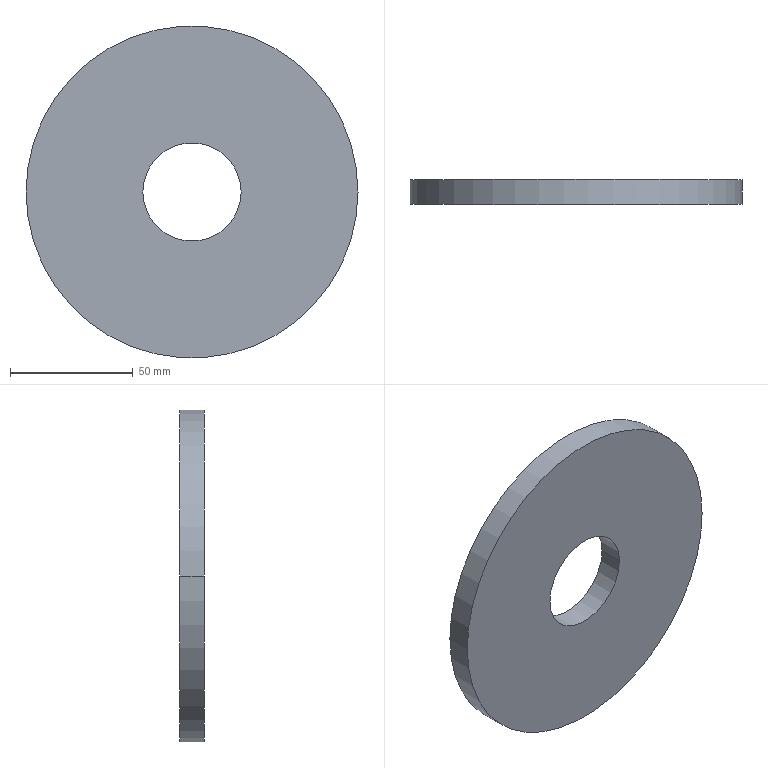Part | SolidWorks | features BaseBody 1 | 1 solid | 6 faces | box 135 x 10 x 135 mm | volume 130572 mm3 | cylinder 4 | plane 2 | commonest cylinder face diameters 40 x2 135 x2
STEP:
#1=CARTESIAN_POINT('',(-2112.95,1114.894,-1577.624));
#2=VERTEX_POINT('',#1);
#3=CARTESIAN_POINT('',(-2112.95,1104.894,-1577.624));
#4=VERTEX_POINT('',#3);
#5=CARTESIAN_POINT('',(-2112.95,1114.894,-1577.624));
#6=DIRECTION('',(0.,-1.,0.));
#7=VECTOR('',#6,1000.);
#8=LINE('',#5,#7);
#9=EDGE_CURVE('',#2,#4,#8,.T.);
#10=ORIENTED_EDGE('',*,*,#9,.F.);
#11=CARTESIAN_POINT('',(-2152.95,1114.894,-1577.624));
#12=VERTEX_POINT('',#11);
#13=CARTESIAN_POINT('',(-2132.95,1114.894,-1577.624));
#14=DIRECTION('',(0.,1.,0.));
#15=DIRECTION('',(1.,0.,0.));
#16=AXIS2_PLACEMENT_3D('',#13,#14,#15);
#17=CIRCLE('',#16,20.);
#18=EDGE_CURVE('',#2,#12,#17,.T.);
#19=ORIENTED_EDGE('',*,*,#18,.T.);
#20=CARTESIAN_POINT('',(-2152.95,1104.894,-1577.624));
#21=VERTEX_POINT('',#20);
#22=CARTESIAN_POINT('',(-2152.95,1114.894,-1577.624));
#23=DIRECTION('',(0.,-1.,0.));
#24=VECTOR('',#23,1000.);
#25=LINE('',#22,#24);
#26=EDGE_CURVE('',#12,#21,#25,.T.);
#27=ORIENTED_EDGE('',*,*,#26,.T.);
#28=CARTESIAN_POINT('',(-2132.95,1104.894,-1577.624));
#29=DIRECTION('',(0.,-1.,0.));
#30=DIRECTION('',(-1.,0.,0.));
#31=AXIS2_PLACEMENT_3D('',#28,#29,#30);
#32=CIRCLE('',#31,20.);
#33=EDGE_CURVE('',#21,#4,#32,.T.);
#34=ORIENTED_EDGE('',*,*,#33,.T.);
#35=EDGE_LOOP('',(#10,#19,#27,#34));
#36=FACE_OUTER_BOUND('',#35,.T.);
#37=CARTESIAN_POINT('',(-2132.95,1114.894,-1577.624));
#38=DIRECTION('',(0.,1.,0.));
#39=DIRECTION('',(1.,0.,0.));
#40=AXIS2_PLACEMENT_3D('',#37,#38,#39);
#41=CYLINDRICAL_SURFACE('',#40,20.);
#42=ADVANCED_FACE('',(#36),#41,.F.);
#43=CARTESIAN_POINT('',(-2065.45,1104.894,-1577.624));
#44=VERTEX_POINT('',#43);
#45=CARTESIAN_POINT('',(-2065.45,1114.894,-1577.624));
#46=VERTEX_POINT('',#45);
#47=CARTESIAN_POINT('',(-2065.45,1104.894,-1577.624));
#48=DIRECTION('',(0.,1.,0.));
#49=VECTOR('',#48,1000.);
#50=LINE('',#47,#49);
#51=EDGE_CURVE('',#44,#46,#50,.T.);
#52=ORIENTED_EDGE('',*,*,#51,.F.);
#53=CARTESIAN_POINT('',(-2200.45,1104.894,-1577.624));
#54=VERTEX_POINT('',#53);
#55=CARTESIAN_POINT('',(-2132.95,1104.894,-1577.624));
#56=DIRECTION('',(0.,-1.,0.));
#57=DIRECTION('',(-1.,0.,0.));
#58=AXIS2_PLACEMENT_3D('',#55,#56,#57);
#59=CIRCLE('',#58,67.5);
#60=EDGE_CURVE('',#54,#44,#59,.T.);
#61=ORIENTED_EDGE('',*,*,#60,.F.);
#62=CARTESIAN_POINT('',(-2200.45,1114.894,-1577.624));
#63=VERTEX_POINT('',#62);
#64=CARTESIAN_POINT('',(-2200.45,1104.894,-1577.624));
#65=DIRECTION('',(0.,1.,0.));
#66=VECTOR('',#65,1000.);
#67=LINE('',#64,#66);
#68=EDGE_CURVE('',#54,#63,#67,.T.);
#69=ORIENTED_EDGE('',*,*,#68,.T.);
#70=CARTESIAN_POINT('',(-2132.95,1114.894,-1577.624));
#71=DIRECTION('',(0.,1.,0.));
#72=DIRECTION('',(1.,0.,0.));
#73=AXIS2_PLACEMENT_3D('',#70,#71,#72);
#74=CIRCLE('',#73,67.5);
#75=EDGE_CURVE('',#46,#63,#74,.T.);
#76=ORIENTED_EDGE('',*,*,#75,.F.);
#77=EDGE_LOOP('',(#52,#61,#69,#76));
#78=FACE_OUTER_BOUND('',#77,.T.);
#79=CARTESIAN_POINT('',(-2132.95,1104.894,-1577.624));
#80=DIRECTION('',(0.,1.,0.));
#81=DIRECTION('',(1.,0.,0.));
#82=AXIS2_PLACEMENT_3D('',#79,#80,#81);
#83=CYLINDRICAL_SURFACE('',#82,67.5);
#84=ADVANCED_FACE('',(#78),#83,.T.);
#85=ORIENTED_EDGE('',*,*,#33,.F.);
#86=CARTESIAN_POINT('',(-2132.95,1104.894,-1577.624));
#87=DIRECTION('',(0.,-1.,0.));
#88=DIRECTION('',(1.,0.,0.));
#89=AXIS2_PLACEMENT_3D('',#86,#87,#88);
#90=CIRCLE('',#89,20.);
#91=EDGE_CURVE('',#4,#21,#90,.T.);
#92=ORIENTED_EDGE('',*,*,#91,.F.);
#93=EDGE_LOOP('',(#85,#92));
#94=FACE_BOUND('',#93,.T.);
#95=ORIENTED_EDGE('',*,*,#60,.T.);
#96=CARTESIAN_POINT('',(-2132.95,1104.894,-1577.624));
#97=DIRECTION('',(0.,-1.,0.));
#98=DIRECTION('',(1.,0.,0.));
#99=AXIS2_PLACEMENT_3D('',#96,#97,#98);
#100=CIRCLE('',#99,67.5);
#101=EDGE_CURVE('',#44,#54,#100,.T.);
#102=ORIENTED_EDGE('',*,*,#101,.T.);
#103=EDGE_LOOP('',(#95,#102));
#104=FACE_OUTER_BOUND('',#103,.T.);
#105=CARTESIAN_POINT('',(-2064.1,1104.894,-1646.474));
#106=DIRECTION('',(0.,-1.,0.));
#107=DIRECTION('',(0.,0.,-1.));
#108=AXIS2_PLACEMENT_3D('',#105,#106,#107);
#109=PLANE('',#108);
#110=ADVANCED_FACE('',(#94,#104),#109,.T.);
#111=ORIENTED_EDGE('',*,*,#91,.T.);
#112=ORIENTED_EDGE('',*,*,#26,.F.);
#113=CARTESIAN_POINT('',(-2132.95,1114.894,-1577.624));
#114=DIRECTION('',(0.,1.,0.));
#115=DIRECTION('',(-1.,0.,0.));
#116=AXIS2_PLACEMENT_3D('',#113,#114,#115);
#117=CIRCLE('',#116,20.);
#118=EDGE_CURVE('',#12,#2,#117,.T.);
#119=ORIENTED_EDGE('',*,*,#118,.T.);
#120=ORIENTED_EDGE('',*,*,#9,.T.);
#121=EDGE_LOOP('',(#111,#112,#119,#120));
#122=FACE_OUTER_BOUND('',#121,.T.);
#123=CARTESIAN_POINT('',(-2132.95,1114.894,-1577.624));
#124=DIRECTION('',(0.,1.,0.));
#125=DIRECTION('',(-1.,0.,0.));
#126=AXIS2_PLACEMENT_3D('',#123,#124,#125);
#127=CYLINDRICAL_SURFACE('',#126,20.);
#128=ADVANCED_FACE('',(#122),#127,.F.);
#129=ORIENTED_EDGE('',*,*,#18,.F.);
#130=ORIENTED_EDGE('',*,*,#118,.F.);
#131=EDGE_LOOP('',(#129,#130));
#132=FACE_BOUND('',#131,.T.);
#133=ORIENTED_EDGE('',*,*,#75,.T.);
#134=CARTESIAN_POINT('',(-2132.95,1114.894,-1577.624));
#135=DIRECTION('',(0.,1.,0.));
#136=DIRECTION('',(-1.,0.,0.));
#137=AXIS2_PLACEMENT_3D('',#134,#135,#136);
#138=CIRCLE('',#137,67.5);
#139=EDGE_CURVE('',#63,#46,#138,.T.);
#140=ORIENTED_EDGE('',*,*,#139,.T.);
#141=EDGE_LOOP('',(#133,#140));
#142=FACE_OUTER_BOUND('',#141,.T.);
#143=CARTESIAN_POINT('',(-2064.1,1114.894,-1508.774));
#144=DIRECTION('',(0.,1.,0.));
#145=DIRECTION('',(1.,0.,0.));
#146=AXIS2_PLACEMENT_3D('',#143,#144,#145);
#147=PLANE('',#146);
#148=ADVANCED_FACE('',(#132,#142),#147,.T.);
#149=ORIENTED_EDGE('',*,*,#139,.F.);
#150=ORIENTED_EDGE('',*,*,#68,.F.);
#151=ORIENTED_EDGE('',*,*,#101,.F.);
#152=ORIENTED_EDGE('',*,*,#51,.T.);
#153=EDGE_LOOP('',(#149,#150,#151,#152));
#154=FACE_OUTER_BOUND('',#153,.T.);
#155=CARTESIAN_POINT('',(-2132.95,1104.894,-1577.624));
#156=DIRECTION('',(0.,1.,0.));
#157=DIRECTION('',(-1.,0.,0.));
#158=AXIS2_PLACEMENT_3D('',#155,#156,#157);
#159=CYLINDRICAL_SURFACE('',#158,67.5);
#160=ADVANCED_FACE('',(#154),#159,.T.);
#161=CLOSED_SHELL('',(#42,#84,#110,#128,#148,#160));
#162=MANIFOLD_SOLID_BREP('',#161);
#163=CARTESIAN_POINT('',(0.,0.,0.));
#164=DIRECTION('',(0.,0.,1.));
#165=DIRECTION('',(1.,0.,0.));
#166=AXIS2_PLACEMENT_3D('',#163,#164,#165);
#167=(LENGTH_UNIT()NAMED_UNIT(*)SI_UNIT(.MILLI.,.METRE.));
#168=UNCERTAINTY_MEASURE_WITH_UNIT(LENGTH_MEASURE(0.00001),#167,'','');
#169=(NAMED_UNIT(*)PLANE_ANGLE_UNIT()SI_UNIT($,.RADIAN.));
#170=(NAMED_UNIT(*)SI_UNIT($,.STERADIAN.)SOLID_ANGLE_UNIT());
#171=(GEOMETRIC_REPRESENTATION_CONTEXT(3)GLOBAL_UNCERTAINTY_ASSIGNED_CONTEXT((#168))GLOBAL_UNIT_ASSIGNED_CONTEXT((#167,#169,#170))REPRESENTATION_CONTEXT('',''));
#172=ADVANCED_BREP_SHAPE_REPRESENTATION('',(#162,#166),#171);